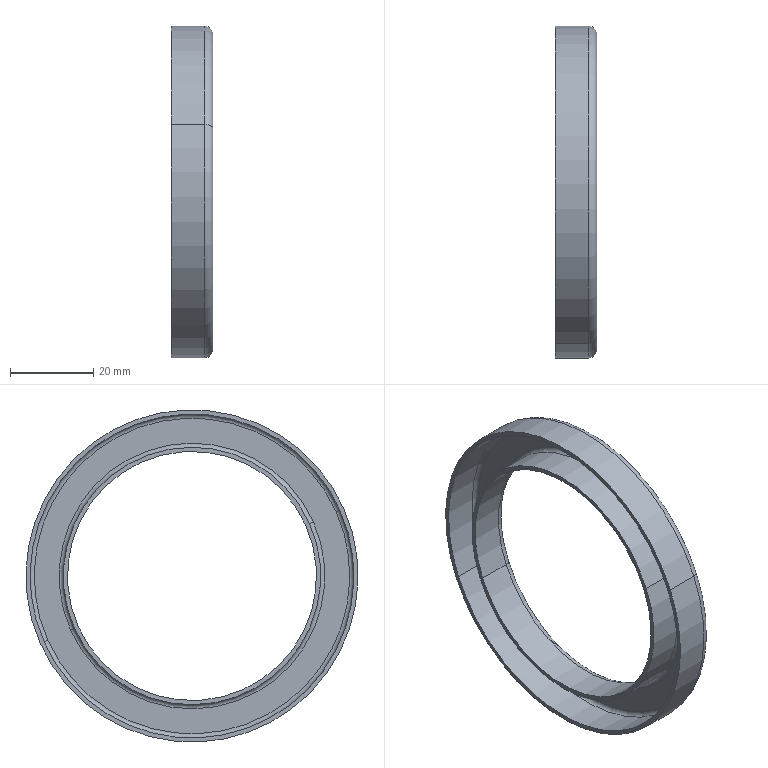Part | STEP file | Input 65 | 1 solid | 20 faces | box 10 x 80 x 80 mm | volume 5874 mm3 | cylinder 8 | torus 8 | plane 4 | commonest cylinder face diameters 60 x2 62 x2 78 x2 80 x2
STEP:
#1=CARTESIAN_POINT('',(0.,0.,0.));
#2=DIRECTION('',(0.,0.,1.));
#3=DIRECTION('',(1.,0.,0.));
#4=AXIS2_PLACEMENT_3D('',#1,#2,#3);
#5=CARTESIAN_POINT('',(4135.,-28.311,12.628));
#6=VERTEX_POINT('',#5);
#7=CARTESIAN_POINT('',(4135.,28.311,-12.628));
#8=VERTEX_POINT('',#7);
#9=CARTESIAN_POINT('',(4135.,0.,0.));
#10=DIRECTION('',(-1.,0.,0.));
#11=DIRECTION('',(0.,-0.9133,0.4074));
#12=AXIS2_PLACEMENT_3D('',#9,#10,#11);
#13=CIRCLE('',#12,31.);
#14=CARTESIAN_POINT('',(4127.,0.,0.));
#15=DIRECTION('',(-1.,0.,0.));
#16=DIRECTION('',(0.,-0.9133,0.4074));
#17=AXIS2_PLACEMENT_3D('',#14,#15,#16);
#18=CYLINDRICAL_SURFACE('',#17,31.);
#19=CARTESIAN_POINT('',(0.,-8.));
#20=DIRECTION('',(1.,0.));
#21=VECTOR('',#20,1.);
#22=LINE('',#19,#21);
#23=(GEOMETRIC_REPRESENTATION_CONTEXT(2)PARAMETRIC_REPRESENTATION_CONTEXT()REPRESENTATION_CONTEXT('',''));
#24=DEFINITIONAL_REPRESENTATION('',(#22),#23);
#25=PCURVE('',#18,#24);
#26=CARTESIAN_POINT('',(4135.,0.,0.));
#27=DIRECTION('',(-1.,0.,0.));
#28=DIRECTION('',(0.,-0.9133,0.4074));
#29=AXIS2_PLACEMENT_3D('',#26,#27,#28);
#30=TOROIDAL_SURFACE('',#29,32.,1.);
#31=CARTESIAN_POINT('',(0.,3.142));
#32=DIRECTION('',(1.,0.));
#33=VECTOR('',#32,1.);
#34=LINE('',#31,#33);
#35=(GEOMETRIC_REPRESENTATION_CONTEXT(2)PARAMETRIC_REPRESENTATION_CONTEXT()REPRESENTATION_CONTEXT('',''));
#36=DEFINITIONAL_REPRESENTATION('',(#34),#35);
#37=PCURVE('',#30,#36);
#38=SURFACE_CURVE('',#13,(#25,#37),.PCURVE_S1.);
#39=EDGE_CURVE('',#6,#8,#38,.T.);
#40=ORIENTED_EDGE('',*,*,#39,.T.);
#41=CARTESIAN_POINT('',(4127.,28.311,-12.628));
#42=VERTEX_POINT('',#41);
#43=CARTESIAN_POINT('',(4127.,28.311,-12.628));
#44=DIRECTION('',(-1.,0.,0.));
#45=VECTOR('',#44,1.);
#46=LINE('',#43,#45);
#47=CARTESIAN_POINT('',(3.142,0.));
#48=DIRECTION('',(0.,1.));
#49=VECTOR('',#48,1.);
#50=LINE('',#47,#49);
#51=(GEOMETRIC_REPRESENTATION_CONTEXT(2)PARAMETRIC_REPRESENTATION_CONTEXT()REPRESENTATION_CONTEXT('',''));
#52=DEFINITIONAL_REPRESENTATION('',(#50),#51);
#53=PCURVE('',#18,#52);
#54=CARTESIAN_POINT('',(4127.,0.,0.));
#55=DIRECTION('',(-1.,0.,0.));
#56=DIRECTION('',(0.,-0.9133,0.4074));
#57=AXIS2_PLACEMENT_3D('',#54,#55,#56);
#58=CYLINDRICAL_SURFACE('',#57,31.);
#59=CARTESIAN_POINT('',(3.142,0.));
#60=DIRECTION('',(0.,1.));
#61=VECTOR('',#60,1.);
#62=LINE('',#59,#61);
#63=(GEOMETRIC_REPRESENTATION_CONTEXT(2)PARAMETRIC_REPRESENTATION_CONTEXT()REPRESENTATION_CONTEXT('',''));
#64=DEFINITIONAL_REPRESENTATION('',(#62),#63);
#65=PCURVE('',#58,#64);
#66=SURFACE_CURVE('',#46,(#53,#65),.PCURVE_S1.);
#67=EDGE_CURVE('',#8,#42,#66,.T.);
#68=ORIENTED_EDGE('',*,*,#67,.T.);
#69=CARTESIAN_POINT('',(4127.,-28.311,12.628));
#70=VERTEX_POINT('',#69);
#71=CARTESIAN_POINT('',(4127.,0.,0.));
#72=DIRECTION('',(-1.,0.,0.));
#73=DIRECTION('',(0.,-0.9133,0.4074));
#74=AXIS2_PLACEMENT_3D('',#71,#72,#73);
#75=CIRCLE('',#74,31.);
#76=CARTESIAN_POINT('',(0.,0.));
#77=DIRECTION('',(1.,0.));
#78=VECTOR('',#77,1.);
#79=LINE('',#76,#78);
#80=(GEOMETRIC_REPRESENTATION_CONTEXT(2)PARAMETRIC_REPRESENTATION_CONTEXT()REPRESENTATION_CONTEXT('',''));
#81=DEFINITIONAL_REPRESENTATION('',(#79),#80);
#82=PCURVE('',#18,#81);
#83=CARTESIAN_POINT('',(4127.,-28.311,12.628));
#84=DIRECTION('',(-1.,0.,0.));
#85=DIRECTION('',(0.,-0.9133,0.4074));
#86=AXIS2_PLACEMENT_3D('',#83,#84,#85);
#87=PLANE('',#86);
#88=CARTESIAN_POINT('',(-31.,0.));
#89=DIRECTION('',(1.,0.));
#90=AXIS2_PLACEMENT_2D('',#88,#89);
#91=CIRCLE('',#90,31.);
#92=(GEOMETRIC_REPRESENTATION_CONTEXT(2)PARAMETRIC_REPRESENTATION_CONTEXT()REPRESENTATION_CONTEXT('',''));
#93=DEFINITIONAL_REPRESENTATION('',(#91),#92);
#94=PCURVE('',#87,#93);
#95=SURFACE_CURVE('',#75,(#82,#94),.PCURVE_S1.);
#96=EDGE_CURVE('',#70,#42,#95,.T.);
#97=ORIENTED_EDGE('',*,*,#96,.F.);
#98=CARTESIAN_POINT('',(4127.,-28.311,12.628));
#99=DIRECTION('',(-1.,0.,0.));
#100=VECTOR('',#99,1.);
#101=LINE('',#98,#100);
#102=CARTESIAN_POINT('',(0.,0.));
#103=DIRECTION('',(0.,1.));
#104=VECTOR('',#103,1.);
#105=LINE('',#102,#104);
#106=(GEOMETRIC_REPRESENTATION_CONTEXT(2)PARAMETRIC_REPRESENTATION_CONTEXT()REPRESENTATION_CONTEXT('',''));
#107=DEFINITIONAL_REPRESENTATION('',(#105),#106);
#108=PCURVE('',#18,#107);
#109=CARTESIAN_POINT('',(6.283,0.));
#110=DIRECTION('',(0.,1.));
#111=VECTOR('',#110,1.);
#112=LINE('',#109,#111);
#113=(GEOMETRIC_REPRESENTATION_CONTEXT(2)PARAMETRIC_REPRESENTATION_CONTEXT()REPRESENTATION_CONTEXT('',''));
#114=DEFINITIONAL_REPRESENTATION('',(#112),#113);
#115=PCURVE('',#58,#114);
#116=SURFACE_CURVE('',#101,(#108,#115),.PCURVE_S1.);
#117=EDGE_CURVE('',#6,#70,#116,.T.);
#118=ORIENTED_EDGE('',*,*,#117,.F.);
#119=EDGE_LOOP('',(#40,#68,#97,#118));
#120=FACE_BOUND('',#119,.T.);
#121=ADVANCED_FACE('',(#120),#18,.T.);
#122=CARTESIAN_POINT('',(4136.,-29.225,13.036));
#123=VERTEX_POINT('',#122);
#124=CARTESIAN_POINT('',(4135.,-29.225,13.036));
#125=DIRECTION('',(0.,-0.4074,-0.9133));
#126=DIRECTION('',(0.,0.9133,-0.4074));
#127=AXIS2_PLACEMENT_3D('',#124,#125,#126);
#128=CIRCLE('',#127,1.);
#129=CARTESIAN_POINT('',(4135.,0.,0.));
#130=DIRECTION('',(-1.,0.,0.));
#131=DIRECTION('',(0.,-0.9133,0.4074));
#132=AXIS2_PLACEMENT_3D('',#129,#130,#131);
#133=TOROIDAL_SURFACE('',#132,32.,1.);
#134=CARTESIAN_POINT('',(6.283,3.142));
#135=DIRECTION('',(0.,1.));
#136=VECTOR('',#135,1.);
#137=LINE('',#134,#136);
#138=(GEOMETRIC_REPRESENTATION_CONTEXT(2)PARAMETRIC_REPRESENTATION_CONTEXT()REPRESENTATION_CONTEXT('',''));
#139=DEFINITIONAL_REPRESENTATION('',(#137),#138);
#140=PCURVE('',#133,#139);
#141=CARTESIAN_POINT('',(0.,3.142));
#142=DIRECTION('',(0.,1.));
#143=VECTOR('',#142,1.);
#144=LINE('',#141,#143);
#145=(GEOMETRIC_REPRESENTATION_CONTEXT(2)PARAMETRIC_REPRESENTATION_CONTEXT()REPRESENTATION_CONTEXT('',''));
#146=DEFINITIONAL_REPRESENTATION('',(#144),#145);
#147=PCURVE('',#30,#146);
#148=SURFACE_CURVE('',#128,(#140,#147),.PCURVE_S1.);
#149=EDGE_CURVE('',#6,#123,#148,.T.);
#150=ORIENTED_EDGE('',*,*,#149,.T.);
#151=CARTESIAN_POINT('',(4136.,29.225,-13.036));
#152=VERTEX_POINT('',#151);
#153=CARTESIAN_POINT('',(4136.,0.,0.));
#154=DIRECTION('',(-1.,0.,0.));
#155=DIRECTION('',(0.,-0.9133,0.4074));
#156=AXIS2_PLACEMENT_3D('',#153,#154,#155);
#157=CIRCLE('',#156,32.);
#158=CARTESIAN_POINT('',(0.,4.712));
#159=DIRECTION('',(1.,0.));
#160=VECTOR('',#159,1.);
#161=LINE('',#158,#160);
#162=(GEOMETRIC_REPRESENTATION_CONTEXT(2)PARAMETRIC_REPRESENTATION_CONTEXT()REPRESENTATION_CONTEXT('',''));
#163=DEFINITIONAL_REPRESENTATION('',(#161),#162);
#164=PCURVE('',#133,#163);
#165=CARTESIAN_POINT('',(4136.,-34.704,15.48));
#166=DIRECTION('',(-1.,0.,0.));
#167=DIRECTION('',(0.,-0.9133,0.4074));
#168=AXIS2_PLACEMENT_3D('',#165,#166,#167);
#169=PLANE('',#168);
#170=CARTESIAN_POINT('',(-38.,0.));
#171=DIRECTION('',(1.,0.));
#172=AXIS2_PLACEMENT_2D('',#170,#171);
#173=CIRCLE('',#172,32.);
#174=(GEOMETRIC_REPRESENTATION_CONTEXT(2)PARAMETRIC_REPRESENTATION_CONTEXT()REPRESENTATION_CONTEXT('',''));
#175=DEFINITIONAL_REPRESENTATION('',(#173),#174);
#176=PCURVE('',#169,#175);
#177=SURFACE_CURVE('',#157,(#164,#176),.PCURVE_S1.);
#178=EDGE_CURVE('',#152,#123,#177,.T.);
#179=ORIENTED_EDGE('',*,*,#178,.F.);
#180=CARTESIAN_POINT('',(4135.,29.225,-13.036));
#181=DIRECTION('',(0.,0.4074,0.9133));
#182=DIRECTION('',(0.,-0.9133,0.4074));
#183=AXIS2_PLACEMENT_3D('',#180,#181,#182);
#184=CIRCLE('',#183,1.);
#185=CARTESIAN_POINT('',(3.142,3.142));
#186=DIRECTION('',(0.,1.));
#187=VECTOR('',#186,1.);
#188=LINE('',#185,#187);
#189=(GEOMETRIC_REPRESENTATION_CONTEXT(2)PARAMETRIC_REPRESENTATION_CONTEXT()REPRESENTATION_CONTEXT('',''));
#190=DEFINITIONAL_REPRESENTATION('',(#188),#189);
#191=PCURVE('',#133,#190);
#192=CARTESIAN_POINT('',(3.142,3.142));
#193=DIRECTION('',(0.,1.));
#194=VECTOR('',#193,1.);
#195=LINE('',#192,#194);
#196=(GEOMETRIC_REPRESENTATION_CONTEXT(2)PARAMETRIC_REPRESENTATION_CONTEXT()REPRESENTATION_CONTEXT('',''));
#197=DEFINITIONAL_REPRESENTATION('',(#195),#196);
#198=PCURVE('',#30,#197);
#199=SURFACE_CURVE('',#184,(#191,#198),.PCURVE_S1.);
#200=EDGE_CURVE('',#8,#152,#199,.T.);
#201=ORIENTED_EDGE('',*,*,#200,.F.);
#202=CARTESIAN_POINT('',(4135.,0.,0.));
#203=DIRECTION('',(-1.,0.,0.));
#204=DIRECTION('',(0.,-0.9133,0.4074));
#205=AXIS2_PLACEMENT_3D('',#202,#203,#204);
#206=CIRCLE('',#205,31.);
#207=CARTESIAN_POINT('',(0.,3.142));
#208=DIRECTION('',(1.,0.));
#209=VECTOR('',#208,1.);
#210=LINE('',#207,#209);
#211=(GEOMETRIC_REPRESENTATION_CONTEXT(2)PARAMETRIC_REPRESENTATION_CONTEXT()REPRESENTATION_CONTEXT('',''));
#212=DEFINITIONAL_REPRESENTATION('',(#210),#211);
#213=PCURVE('',#133,#212);
#214=CARTESIAN_POINT('',(0.,-8.));
#215=DIRECTION('',(1.,0.));
#216=VECTOR('',#215,1.);
#217=LINE('',#214,#216);
#218=(GEOMETRIC_REPRESENTATION_CONTEXT(2)PARAMETRIC_REPRESENTATION_CONTEXT()REPRESENTATION_CONTEXT('',''));
#219=DEFINITIONAL_REPRESENTATION('',(#217),#218);
#220=PCURVE('',#58,#219);
#221=SURFACE_CURVE('',#206,(#213,#220),.PCURVE_S1.);
#222=EDGE_CURVE('',#8,#6,#221,.T.);
#223=ORIENTED_EDGE('',*,*,#222,.T.);
#224=EDGE_LOOP('',(#150,#179,#201,#223));
#225=FACE_BOUND('',#224,.F.);
#226=ADVANCED_FACE('',(#225),#133,.F.);
#227=CARTESIAN_POINT('',(4136.,-34.704,15.48));
#228=VERTEX_POINT('',#227);
#229=CARTESIAN_POINT('',(4135.,-35.617,15.887));
#230=VERTEX_POINT('',#229);
#231=CARTESIAN_POINT('',(4135.,-34.704,15.48));
#232=DIRECTION('',(0.,-0.4074,-0.9133));
#233=DIRECTION('',(0.,0.9133,-0.4074));
#234=AXIS2_PLACEMENT_3D('',#231,#232,#233);
#235=CIRCLE('',#234,1.);
#236=CARTESIAN_POINT('',(4135.,0.,0.));
#237=DIRECTION('',(-1.,0.,0.));
#238=DIRECTION('',(0.,-0.9133,0.4074));
#239=AXIS2_PLACEMENT_3D('',#236,#237,#238);
#240=TOROIDAL_SURFACE('',#239,38.,1.);
#241=CARTESIAN_POINT('',(6.283,3.142));
#242=DIRECTION('',(0.,1.));
#243=VECTOR('',#242,1.);
#244=LINE('',#241,#243);
#245=(GEOMETRIC_REPRESENTATION_CONTEXT(2)PARAMETRIC_REPRESENTATION_CONTEXT()REPRESENTATION_CONTEXT('',''));
#246=DEFINITIONAL_REPRESENTATION('',(#244),#245);
#247=PCURVE('',#240,#246);
#248=CARTESIAN_POINT('',(4135.,0.,0.));
#249=DIRECTION('',(-1.,0.,0.));
#250=DIRECTION('',(0.,-0.9133,0.4074));
#251=AXIS2_PLACEMENT_3D('',#248,#249,#250);
#252=TOROIDAL_SURFACE('',#251,38.,1.);
#253=CARTESIAN_POINT('',(0.,3.142));
#254=DIRECTION('',(0.,1.));
#255=VECTOR('',#254,1.);
#256=LINE('',#253,#255);
#257=(GEOMETRIC_REPRESENTATION_CONTEXT(2)PARAMETRIC_REPRESENTATION_CONTEXT()REPRESENTATION_CONTEXT('',''));
#258=DEFINITIONAL_REPRESENTATION('',(#256),#257);
#259=PCURVE('',#252,#258);
#260=SURFACE_CURVE('',#235,(#247,#259),.PCURVE_S1.);
#261=EDGE_CURVE('',#228,#230,#260,.T.);
#262=ORIENTED_EDGE('',*,*,#261,.T.);
#263=CARTESIAN_POINT('',(4135.,35.617,-15.887));
#264=VERTEX_POINT('',#263);
#265=CARTESIAN_POINT('',(4135.,0.,0.));
#266=DIRECTION('',(-1.,0.,0.));
#267=DIRECTION('',(0.,-0.9133,0.4074));
#268=AXIS2_PLACEMENT_3D('',#265,#266,#267);
#269=CIRCLE('',#268,39.);
#270=CARTESIAN_POINT('',(0.,6.283));
#271=DIRECTION('',(1.,0.));
#272=VECTOR('',#271,1.);
#273=LINE('',#270,#272);
#274=(GEOMETRIC_REPRESENTATION_CONTEXT(2)PARAMETRIC_REPRESENTATION_CONTEXT()REPRESENTATION_CONTEXT('',''));
#275=DEFINITIONAL_REPRESENTATION('',(#273),#274);
#276=PCURVE('',#240,#275);
#277=CARTESIAN_POINT('',(4127.,0.,0.));
#278=DIRECTION('',(-1.,0.,0.));
#279=DIRECTION('',(0.,-0.9133,0.4074));
#280=AXIS2_PLACEMENT_3D('',#277,#278,#279);
#281=CYLINDRICAL_SURFACE('',#280,39.);
#282=CARTESIAN_POINT('',(0.,-8.));
#283=DIRECTION('',(1.,0.));
#284=VECTOR('',#283,1.);
#285=LINE('',#282,#284);
#286=(GEOMETRIC_REPRESENTATION_CONTEXT(2)PARAMETRIC_REPRESENTATION_CONTEXT()REPRESENTATION_CONTEXT('',''));
#287=DEFINITIONAL_REPRESENTATION('',(#285),#286);
#288=PCURVE('',#281,#287);
#289=SURFACE_CURVE('',#269,(#276,#288),.PCURVE_S1.);
#290=EDGE_CURVE('',#264,#230,#289,.T.);
#291=ORIENTED_EDGE('',*,*,#290,.F.);
#292=CARTESIAN_POINT('',(4136.,34.704,-15.48));
#293=VERTEX_POINT('',#292);
#294=CARTESIAN_POINT('',(4135.,34.704,-15.48));
#295=DIRECTION('',(0.,0.4074,0.9133));
#296=DIRECTION('',(0.,-0.9133,0.4074));
#297=AXIS2_PLACEMENT_3D('',#294,#295,#296);
#298=CIRCLE('',#297,1.);
#299=CARTESIAN_POINT('',(3.142,3.142));
#300=DIRECTION('',(0.,1.));
#301=VECTOR('',#300,1.);
#302=LINE('',#299,#301);
#303=(GEOMETRIC_REPRESENTATION_CONTEXT(2)PARAMETRIC_REPRESENTATION_CONTEXT()REPRESENTATION_CONTEXT('',''));
#304=DEFINITIONAL_REPRESENTATION('',(#302),#303);
#305=PCURVE('',#240,#304);
#306=CARTESIAN_POINT('',(3.142,3.142));
#307=DIRECTION('',(0.,1.));
#308=VECTOR('',#307,1.);
#309=LINE('',#306,#308);
#310=(GEOMETRIC_REPRESENTATION_CONTEXT(2)PARAMETRIC_REPRESENTATION_CONTEXT()REPRESENTATION_CONTEXT('',''));
#311=DEFINITIONAL_REPRESENTATION('',(#309),#310);
#312=PCURVE('',#252,#311);
#313=SURFACE_CURVE('',#298,(#305,#312),.PCURVE_S1.);
#314=EDGE_CURVE('',#293,#264,#313,.T.);
#315=ORIENTED_EDGE('',*,*,#314,.F.);
#316=CARTESIAN_POINT('',(4136.,0.,0.));
#317=DIRECTION('',(-1.,0.,0.));
#318=DIRECTION('',(0.,-0.9133,0.4074));
#319=AXIS2_PLACEMENT_3D('',#316,#317,#318);
#320=CIRCLE('',#319,38.);
#321=CARTESIAN_POINT('',(0.,4.712));
#322=DIRECTION('',(1.,0.));
#323=VECTOR('',#322,1.);
#324=LINE('',#321,#323);
#325=(GEOMETRIC_REPRESENTATION_CONTEXT(2)PARAMETRIC_REPRESENTATION_CONTEXT()REPRESENTATION_CONTEXT('',''));
#326=DEFINITIONAL_REPRESENTATION('',(#324),#325);
#327=PCURVE('',#240,#326);
#328=CARTESIAN_POINT('',(-38.,0.));
#329=DIRECTION('',(1.,0.));
#330=AXIS2_PLACEMENT_2D('',#328,#329);
#331=CIRCLE('',#330,38.);
#332=(GEOMETRIC_REPRESENTATION_CONTEXT(2)PARAMETRIC_REPRESENTATION_CONTEXT()REPRESENTATION_CONTEXT('',''));
#333=DEFINITIONAL_REPRESENTATION('',(#331),#332);
#334=PCURVE('',#169,#333);
#335=SURFACE_CURVE('',#320,(#327,#334),.PCURVE_S1.);
#336=EDGE_CURVE('',#293,#228,#335,.T.);
#337=ORIENTED_EDGE('',*,*,#336,.T.);
#338=EDGE_LOOP('',(#262,#291,#315,#337));
#339=FACE_BOUND('',#338,.F.);
#340=ADVANCED_FACE('',(#339),#240,.F.);
#341=CARTESIAN_POINT('',(4127.,-35.617,15.887));
#342=VERTEX_POINT('',#341);
#343=CARTESIAN_POINT('',(4127.,-35.617,15.887));
#344=DIRECTION('',(-1.,0.,0.));
#345=VECTOR('',#344,1.);
#346=LINE('',#343,#345);
#347=CARTESIAN_POINT('',(6.283,0.));
#348=DIRECTION('',(0.,1.));
#349=VECTOR('',#348,1.);
#350=LINE('',#347,#349);
#351=(GEOMETRIC_REPRESENTATION_CONTEXT(2)PARAMETRIC_REPRESENTATION_CONTEXT()REPRESENTATION_CONTEXT('',''));
#352=DEFINITIONAL_REPRESENTATION('',(#350),#351);
#353=PCURVE('',#281,#352);
#354=CARTESIAN_POINT('',(4127.,0.,0.));
#355=DIRECTION('',(-1.,0.,0.));
#356=DIRECTION('',(0.,-0.9133,0.4074));
#357=AXIS2_PLACEMENT_3D('',#354,#355,#356);
#358=CYLINDRICAL_SURFACE('',#357,39.);
#359=CARTESIAN_POINT('',(0.,0.));
#360=DIRECTION('',(0.,1.));
#361=VECTOR('',#360,1.);
#362=LINE('',#359,#361);
#363=(GEOMETRIC_REPRESENTATION_CONTEXT(2)PARAMETRIC_REPRESENTATION_CONTEXT()REPRESENTATION_CONTEXT('',''));
#364=DEFINITIONAL_REPRESENTATION('',(#362),#363);
#365=PCURVE('',#358,#364);
#366=SURFACE_CURVE('',#346,(#353,#365),.PCURVE_S1.);
#367=EDGE_CURVE('',#230,#342,#366,.T.);
#368=ORIENTED_EDGE('',*,*,#367,.T.);
#369=CARTESIAN_POINT('',(4127.,35.617,-15.887));
#370=VERTEX_POINT('',#369);
#371=CARTESIAN_POINT('',(4127.,0.,0.));
#372=DIRECTION('',(-1.,0.,0.));
#373=DIRECTION('',(0.,-0.9133,0.4074));
#374=AXIS2_PLACEMENT_3D('',#371,#372,#373);
#375=CIRCLE('',#374,39.);
#376=CARTESIAN_POINT('',(0.,0.));
#377=DIRECTION('',(1.,0.));
#378=VECTOR('',#377,1.);
#379=LINE('',#376,#378);
#380=(GEOMETRIC_REPRESENTATION_CONTEXT(2)PARAMETRIC_REPRESENTATION_CONTEXT()REPRESENTATION_CONTEXT('',''));
#381=DEFINITIONAL_REPRESENTATION('',(#379),#380);
#382=PCURVE('',#281,#381);
#383=CARTESIAN_POINT('',(4127.,-36.531,16.295));
#384=DIRECTION('',(-1.,0.,0.));
#385=DIRECTION('',(0.,-0.9133,0.4074));
#386=AXIS2_PLACEMENT_3D('',#383,#384,#385);
#387=PLANE('',#386);
#388=CARTESIAN_POINT('',(-40.,0.));
#389=DIRECTION('',(1.,0.));
#390=AXIS2_PLACEMENT_2D('',#388,#389);
#391=CIRCLE('',#390,39.);
#392=(GEOMETRIC_REPRESENTATION_CONTEXT(2)PARAMETRIC_REPRESENTATION_CONTEXT()REPRESENTATION_CONTEXT('',''));
#393=DEFINITIONAL_REPRESENTATION('',(#391),#392);
#394=PCURVE('',#387,#393);
#395=SURFACE_CURVE('',#375,(#382,#394),.PCURVE_S1.);
#396=EDGE_CURVE('',#370,#342,#395,.T.);
#397=ORIENTED_EDGE('',*,*,#396,.F.);
#398=CARTESIAN_POINT('',(4127.,35.617,-15.887));
#399=DIRECTION('',(-1.,0.,0.));
#400=VECTOR('',#399,1.);
#401=LINE('',#398,#400);
#402=CARTESIAN_POINT('',(3.142,0.));
#403=DIRECTION('',(0.,1.));
#404=VECTOR('',#403,1.);
#405=LINE('',#402,#404);
#406=(GEOMETRIC_REPRESENTATION_CONTEXT(2)PARAMETRIC_REPRESENTATION_CONTEXT()REPRESENTATION_CONTEXT('',''));
#407=DEFINITIONAL_REPRESENTATION('',(#405),#406);
#408=PCURVE('',#281,#407);
#409=CARTESIAN_POINT('',(3.142,0.));
#410=DIRECTION('',(0.,1.));
#411=VECTOR('',#410,1.);
#412=LINE('',#409,#411);
#413=(GEOMETRIC_REPRESENTATION_CONTEXT(2)PARAMETRIC_REPRESENTATION_CONTEXT()REPRESENTATION_CONTEXT('',''));
#414=DEFINITIONAL_REPRESENTATION('',(#412),#413);
#415=PCURVE('',#358,#414);
#416=SURFACE_CURVE('',#401,(#408,#415),.PCURVE_S1.);
#417=EDGE_CURVE('',#264,#370,#416,.T.);
#418=ORIENTED_EDGE('',*,*,#417,.F.);
#419=ORIENTED_EDGE('',*,*,#290,.T.);
#420=EDGE_LOOP('',(#368,#397,#418,#419));
#421=FACE_BOUND('',#420,.F.);
#422=ADVANCED_FACE('',(#421),#281,.F.);
#423=CARTESIAN_POINT('',(4135.,-36.531,16.295));
#424=VERTEX_POINT('',#423);
#425=CARTESIAN_POINT('',(4135.,36.531,-16.295));
#426=VERTEX_POINT('',#425);
#427=CARTESIAN_POINT('',(4135.,0.,0.));
#428=DIRECTION('',(-1.,0.,0.));
#429=DIRECTION('',(0.,-0.9133,0.4074));
#430=AXIS2_PLACEMENT_3D('',#427,#428,#429);
#431=CIRCLE('',#430,40.);
#432=CARTESIAN_POINT('',(4127.,0.,0.));
#433=DIRECTION('',(-1.,0.,0.));
#434=DIRECTION('',(0.,-0.9133,0.4074));
#435=AXIS2_PLACEMENT_3D('',#432,#433,#434);
#436=CYLINDRICAL_SURFACE('',#435,40.);
#437=CARTESIAN_POINT('',(0.,-8.));
#438=DIRECTION('',(1.,0.));
#439=VECTOR('',#438,1.);
#440=LINE('',#437,#439);
#441=(GEOMETRIC_REPRESENTATION_CONTEXT(2)PARAMETRIC_REPRESENTATION_CONTEXT()REPRESENTATION_CONTEXT('',''));
#442=DEFINITIONAL_REPRESENTATION('',(#440),#441);
#443=PCURVE('',#436,#442);
#444=CARTESIAN_POINT('',(4135.,0.,0.));
#445=DIRECTION('',(-1.,0.,0.));
#446=DIRECTION('',(0.,-0.9133,0.4074));
#447=AXIS2_PLACEMENT_3D('',#444,#445,#446);
#448=TOROIDAL_SURFACE('',#447,38.,2.);
#449=CARTESIAN_POINT('',(0.,6.283));
#450=DIRECTION('',(1.,0.));
#451=VECTOR('',#450,1.);
#452=LINE('',#449,#451);
#453=(GEOMETRIC_REPRESENTATION_CONTEXT(2)PARAMETRIC_REPRESENTATION_CONTEXT()REPRESENTATION_CONTEXT('',''));
#454=DEFINITIONAL_REPRESENTATION('',(#452),#453);
#455=PCURVE('',#448,#454);
#456=SURFACE_CURVE('',#431,(#443,#455),.PCURVE_S1.);
#457=EDGE_CURVE('',#424,#426,#456,.T.);
#458=ORIENTED_EDGE('',*,*,#457,.T.);
#459=CARTESIAN_POINT('',(4127.,36.531,-16.295));
#460=VERTEX_POINT('',#459);
#461=CARTESIAN_POINT('',(4127.,36.531,-16.295));
#462=DIRECTION('',(-1.,0.,0.));
#463=VECTOR('',#462,1.);
#464=LINE('',#461,#463);
#465=CARTESIAN_POINT('',(3.142,0.));
#466=DIRECTION('',(0.,1.));
#467=VECTOR('',#466,1.);
#468=LINE('',#465,#467);
#469=(GEOMETRIC_REPRESENTATION_CONTEXT(2)PARAMETRIC_REPRESENTATION_CONTEXT()REPRESENTATION_CONTEXT('',''));
#470=DEFINITIONAL_REPRESENTATION('',(#468),#469);
#471=PCURVE('',#436,#470);
#472=CARTESIAN_POINT('',(4127.,0.,0.));
#473=DIRECTION('',(-1.,0.,0.));
#474=DIRECTION('',(0.,-0.9133,0.4074));
#475=AXIS2_PLACEMENT_3D('',#472,#473,#474);
#476=CYLINDRICAL_SURFACE('',#475,40.);
#477=CARTESIAN_POINT('',(3.142,0.));
#478=DIRECTION('',(0.,1.));
#479=VECTOR('',#478,1.);
#480=LINE('',#477,#479);
#481=(GEOMETRIC_REPRESENTATION_CONTEXT(2)PARAMETRIC_REPRESENTATION_CONTEXT()REPRESENTATION_CONTEXT('',''));
#482=DEFINITIONAL_REPRESENTATION('',(#480),#481);
#483=PCURVE('',#476,#482);
#484=SURFACE_CURVE('',#464,(#471,#483),.PCURVE_S1.);
#485=EDGE_CURVE('',#426,#460,#484,.T.);
#486=ORIENTED_EDGE('',*,*,#485,.T.);
#487=CARTESIAN_POINT('',(4127.,-36.531,16.295));
#488=VERTEX_POINT('',#487);
#489=CARTESIAN_POINT('',(4127.,0.,0.));
#490=DIRECTION('',(-1.,0.,0.));
#491=DIRECTION('',(0.,-0.9133,0.4074));
#492=AXIS2_PLACEMENT_3D('',#489,#490,#491);
#493=CIRCLE('',#492,40.);
#494=CARTESIAN_POINT('',(0.,0.));
#495=DIRECTION('',(1.,0.));
#496=VECTOR('',#495,1.);
#497=LINE('',#494,#496);
#498=(GEOMETRIC_REPRESENTATION_CONTEXT(2)PARAMETRIC_REPRESENTATION_CONTEXT()REPRESENTATION_CONTEXT('',''));
#499=DEFINITIONAL_REPRESENTATION('',(#497),#498);
#500=PCURVE('',#436,#499);
#501=CARTESIAN_POINT('',(-40.,0.));
#502=DIRECTION('',(1.,0.));
#503=AXIS2_PLACEMENT_2D('',#501,#502);
#504=CIRCLE('',#503,40.);
#505=(GEOMETRIC_REPRESENTATION_CONTEXT(2)PARAMETRIC_REPRESENTATION_CONTEXT()REPRESENTATION_CONTEXT('',''));
#506=DEFINITIONAL_REPRESENTATION('',(#504),#505);
#507=PCURVE('',#387,#506);
#508=SURFACE_CURVE('',#493,(#500,#507),.PCURVE_S1.);
#509=EDGE_CURVE('',#488,#460,#508,.T.);
#510=ORIENTED_EDGE('',*,*,#509,.F.);
#511=CARTESIAN_POINT('',(4127.,-36.531,16.295));
#512=DIRECTION('',(-1.,0.,0.));
#513=VECTOR('',#512,1.);
#514=LINE('',#511,#513);
#515=CARTESIAN_POINT('',(0.,0.));
#516=DIRECTION('',(0.,1.));
#517=VECTOR('',#516,1.);
#518=LINE('',#515,#517);
#519=(GEOMETRIC_REPRESENTATION_CONTEXT(2)PARAMETRIC_REPRESENTATION_CONTEXT()REPRESENTATION_CONTEXT('',''));
#520=DEFINITIONAL_REPRESENTATION('',(#518),#519);
#521=PCURVE('',#436,#520);
#522=CARTESIAN_POINT('',(6.283,0.));
#523=DIRECTION('',(0.,1.));
#524=VECTOR('',#523,1.);
#525=LINE('',#522,#524);
#526=(GEOMETRIC_REPRESENTATION_CONTEXT(2)PARAMETRIC_REPRESENTATION_CONTEXT()REPRESENTATION_CONTEXT('',''));
#527=DEFINITIONAL_REPRESENTATION('',(#525),#526);
#528=PCURVE('',#476,#527);
#529=SURFACE_CURVE('',#514,(#521,#528),.PCURVE_S1.);
#530=EDGE_CURVE('',#424,#488,#529,.T.);
#531=ORIENTED_EDGE('',*,*,#530,.F.);
#532=EDGE_LOOP('',(#458,#486,#510,#531));
#533=FACE_BOUND('',#532,.T.);
#534=ADVANCED_FACE('',(#533),#436,.T.);
#535=CARTESIAN_POINT('',(4137.,-34.704,15.48));
#536=VERTEX_POINT('',#535);
#537=CARTESIAN_POINT('',(4137.,34.704,-15.48));
#538=VERTEX_POINT('',#537);
#539=CARTESIAN_POINT('',(4137.,0.,0.));
#540=DIRECTION('',(-1.,0.,0.));
#541=DIRECTION('',(0.,-0.9133,0.4074));
#542=AXIS2_PLACEMENT_3D('',#539,#540,#541);
#543=CIRCLE('',#542,38.);
#544=CARTESIAN_POINT('',(0.,4.712));
#545=DIRECTION('',(1.,0.));
#546=VECTOR('',#545,1.);
#547=LINE('',#544,#546);
#548=(GEOMETRIC_REPRESENTATION_CONTEXT(2)PARAMETRIC_REPRESENTATION_CONTEXT()REPRESENTATION_CONTEXT('',''));
#549=DEFINITIONAL_REPRESENTATION('',(#547),#548);
#550=PCURVE('',#448,#549);
#551=CARTESIAN_POINT('',(4137.,-29.225,13.036));
#552=DIRECTION('',(1.,0.,0.));
#553=DIRECTION('',(0.,0.9133,-0.4074));
#554=AXIS2_PLACEMENT_3D('',#551,#552,#553);
#555=PLANE('',#554);
#556=CARTESIAN_POINT('',(-6.,0.));
#557=CARTESIAN_POINT('',(-6.,65.818));
#558=CARTESIAN_POINT('',(51.,32.909));
#559=CARTESIAN_POINT('',(108.,0.));
#560=CARTESIAN_POINT('',(51.,-32.909));
#561=CARTESIAN_POINT('',(-6.,-65.818));
#562=CARTESIAN_POINT('',(-6.,0.));
#563=(BOUNDED_CURVE()B_SPLINE_CURVE(2,(#556,#557,#558,#559,#560,#561,#562),.UNSPECIFIED.,.T.,.F.)B_SPLINE_CURVE_WITH_KNOTS((1,2,2,2,2,1),(-2.094,0.,2.094,4.189,6.283,8.378),.UNSPECIFIED.)CURVE()GEOMETRIC_REPRESENTATION_ITEM()RATIONAL_B_SPLINE_CURVE((1.,0.5,1.,0.5,1.,0.5,1.))REPRESENTATION_ITEM(''));
#564=(GEOMETRIC_REPRESENTATION_CONTEXT(2)PARAMETRIC_REPRESENTATION_CONTEXT()REPRESENTATION_CONTEXT('',''));
#565=DEFINITIONAL_REPRESENTATION('',(#563),#564);
#566=PCURVE('',#555,#565);
#567=SURFACE_CURVE('',#543,(#550,#566),.PCURVE_S1.);
#568=EDGE_CURVE('',#536,#538,#567,.T.);
#569=ORIENTED_EDGE('',*,*,#568,.T.);
#570=CARTESIAN_POINT('',(4135.,34.704,-15.48));
#571=DIRECTION('',(0.,0.4074,0.9133));
#572=DIRECTION('',(0.,-0.9133,0.4074));
#573=AXIS2_PLACEMENT_3D('',#570,#571,#572);
#574=CIRCLE('',#573,2.);
#575=CARTESIAN_POINT('',(3.142,3.142));
#576=DIRECTION('',(0.,1.));
#577=VECTOR('',#576,1.);
#578=LINE('',#575,#577);
#579=(GEOMETRIC_REPRESENTATION_CONTEXT(2)PARAMETRIC_REPRESENTATION_CONTEXT()REPRESENTATION_CONTEXT('',''));
#580=DEFINITIONAL_REPRESENTATION('',(#578),#579);
#581=PCURVE('',#448,#580);
#582=CARTESIAN_POINT('',(4135.,0.,0.));
#583=DIRECTION('',(-1.,0.,0.));
#584=DIRECTION('',(0.,-0.9133,0.4074));
#585=AXIS2_PLACEMENT_3D('',#582,#583,#584);
#586=TOROIDAL_SURFACE('',#585,38.,2.);
#587=CARTESIAN_POINT('',(3.142,3.142));
#588=DIRECTION('',(0.,1.));
#589=VECTOR('',#588,1.);
#590=LINE('',#587,#589);
#591=(GEOMETRIC_REPRESENTATION_CONTEXT(2)PARAMETRIC_REPRESENTATION_CONTEXT()REPRESENTATION_CONTEXT('',''));
#592=DEFINITIONAL_REPRESENTATION('',(#590),#591);
#593=PCURVE('',#586,#592);
#594=SURFACE_CURVE('',#574,(#581,#593),.PCURVE_S1.);
#595=EDGE_CURVE('',#538,#426,#594,.T.);
#596=ORIENTED_EDGE('',*,*,#595,.T.);
#597=ORIENTED_EDGE('',*,*,#457,.F.);
#598=CARTESIAN_POINT('',(4135.,-34.704,15.48));
#599=DIRECTION('',(0.,-0.4074,-0.9133));
#600=DIRECTION('',(0.,0.9133,-0.4074));
#601=AXIS2_PLACEMENT_3D('',#598,#599,#600);
#602=CIRCLE('',#601,2.);
#603=CARTESIAN_POINT('',(0.,3.142));
#604=DIRECTION('',(0.,1.));
#605=VECTOR('',#604,1.);
#606=LINE('',#603,#605);
#607=(GEOMETRIC_REPRESENTATION_CONTEXT(2)PARAMETRIC_REPRESENTATION_CONTEXT()REPRESENTATION_CONTEXT('',''));
#608=DEFINITIONAL_REPRESENTATION('',(#606),#607);
#609=PCURVE('',#448,#608);
#610=CARTESIAN_POINT('',(6.283,3.142));
#611=DIRECTION('',(0.,1.));
#612=VECTOR('',#611,1.);
#613=LINE('',#610,#612);
#614=(GEOMETRIC_REPRESENTATION_CONTEXT(2)PARAMETRIC_REPRESENTATION_CONTEXT()REPRESENTATION_CONTEXT('',''));
#615=DEFINITIONAL_REPRESENTATION('',(#613),#614);
#616=PCURVE('',#586,#615);
#617=SURFACE_CURVE('',#602,(#609,#616),.PCURVE_S1.);
#618=EDGE_CURVE('',#536,#424,#617,.T.);
#619=ORIENTED_EDGE('',*,*,#618,.F.);
#620=EDGE_LOOP('',(#569,#596,#597,#619));
#621=FACE_BOUND('',#620,.T.);
#622=ADVANCED_FACE('',(#621),#448,.T.);
#623=CARTESIAN_POINT('',(4135.,-27.398,12.221));
#624=VERTEX_POINT('',#623);
#625=CARTESIAN_POINT('',(4135.,27.398,-12.221));
#626=VERTEX_POINT('',#625);
#627=CARTESIAN_POINT('',(4135.,0.,0.));
#628=DIRECTION('',(-1.,0.,0.));
#629=DIRECTION('',(0.,-0.9133,0.4074));
#630=AXIS2_PLACEMENT_3D('',#627,#628,#629);
#631=CIRCLE('',#630,30.);
#632=CARTESIAN_POINT('',(4135.,0.,0.));
#633=DIRECTION('',(-1.,0.,0.));
#634=DIRECTION('',(0.,-0.9133,0.4074));
#635=AXIS2_PLACEMENT_3D('',#632,#633,#634);
#636=TOROIDAL_SURFACE('',#635,32.,2.);
#637=CARTESIAN_POINT('',(0.,3.142));
#638=DIRECTION('',(1.,0.));
#639=VECTOR('',#638,1.);
#640=LINE('',#637,#639);
#641=(GEOMETRIC_REPRESENTATION_CONTEXT(2)PARAMETRIC_REPRESENTATION_CONTEXT()REPRESENTATION_CONTEXT('',''));
#642=DEFINITIONAL_REPRESENTATION('',(#640),#641);
#643=PCURVE('',#636,#642);
#644=CARTESIAN_POINT('',(4127.,0.,0.));
#645=DIRECTION('',(-1.,0.,0.));
#646=DIRECTION('',(0.,-0.9133,0.4074));
#647=AXIS2_PLACEMENT_3D('',#644,#645,#646);
#648=CYLINDRICAL_SURFACE('',#647,30.);
#649=CARTESIAN_POINT('',(0.,-8.));
#650=DIRECTION('',(1.,0.));
#651=VECTOR('',#650,1.);
#652=LINE('',#649,#651);
#653=(GEOMETRIC_REPRESENTATION_CONTEXT(2)PARAMETRIC_REPRESENTATION_CONTEXT()REPRESENTATION_CONTEXT('',''));
#654=DEFINITIONAL_REPRESENTATION('',(#652),#653);
#655=PCURVE('',#648,#654);
#656=SURFACE_CURVE('',#631,(#643,#655),.PCURVE_S1.);
#657=EDGE_CURVE('',#624,#626,#656,.T.);
#658=ORIENTED_EDGE('',*,*,#657,.T.);
#659=CARTESIAN_POINT('',(4137.,29.225,-13.036));
#660=VERTEX_POINT('',#659);
#661=CARTESIAN_POINT('',(4135.,29.225,-13.036));
#662=DIRECTION('',(0.,0.4074,0.9133));
#663=DIRECTION('',(0.,-0.9133,0.4074));
#664=AXIS2_PLACEMENT_3D('',#661,#662,#663);
#665=CIRCLE('',#664,2.);
#666=CARTESIAN_POINT('',(3.142,3.142));
#667=DIRECTION('',(0.,1.));
#668=VECTOR('',#667,1.);
#669=LINE('',#666,#668);
#670=(GEOMETRIC_REPRESENTATION_CONTEXT(2)PARAMETRIC_REPRESENTATION_CONTEXT()REPRESENTATION_CONTEXT('',''));
#671=DEFINITIONAL_REPRESENTATION('',(#669),#670);
#672=PCURVE('',#636,#671);
#673=CARTESIAN_POINT('',(4135.,0.,0.));
#674=DIRECTION('',(-1.,0.,0.));
#675=DIRECTION('',(0.,-0.9133,0.4074));
#676=AXIS2_PLACEMENT_3D('',#673,#674,#675);
#677=TOROIDAL_SURFACE('',#676,32.,2.);
#678=CARTESIAN_POINT('',(3.142,3.142));
#679=DIRECTION('',(0.,1.));
#680=VECTOR('',#679,1.);
#681=LINE('',#678,#680);
#682=(GEOMETRIC_REPRESENTATION_CONTEXT(2)PARAMETRIC_REPRESENTATION_CONTEXT()REPRESENTATION_CONTEXT('',''));
#683=DEFINITIONAL_REPRESENTATION('',(#681),#682);
#684=PCURVE('',#677,#683);
#685=SURFACE_CURVE('',#665,(#672,#684),.PCURVE_S1.);
#686=EDGE_CURVE('',#626,#660,#685,.T.);
#687=ORIENTED_EDGE('',*,*,#686,.T.);
#688=CARTESIAN_POINT('',(4137.,-29.225,13.036));
#689=VERTEX_POINT('',#688);
#690=CARTESIAN_POINT('',(4137.,0.,0.));
#691=DIRECTION('',(-1.,0.,0.));
#692=DIRECTION('',(0.,-0.9133,0.4074));
#693=AXIS2_PLACEMENT_3D('',#690,#691,#692);
#694=CIRCLE('',#693,32.);
#695=CARTESIAN_POINT('',(0.,4.712));
#696=DIRECTION('',(1.,0.));
#697=VECTOR('',#696,1.);
#698=LINE('',#695,#697);
#699=(GEOMETRIC_REPRESENTATION_CONTEXT(2)PARAMETRIC_REPRESENTATION_CONTEXT()REPRESENTATION_CONTEXT('',''));
#700=DEFINITIONAL_REPRESENTATION('',(#698),#699);
#701=PCURVE('',#636,#700);
#702=CARTESIAN_POINT('',(0.,0.));
#703=CARTESIAN_POINT('',(0.,55.426));
#704=CARTESIAN_POINT('',(48.,27.713));
#705=CARTESIAN_POINT('',(96.,0.));
#706=CARTESIAN_POINT('',(48.,-27.713));
#707=CARTESIAN_POINT('',(0.,-55.426));
#708=CARTESIAN_POINT('',(0.,0.));
#709=(BOUNDED_CURVE()B_SPLINE_CURVE(2,(#702,#703,#704,#705,#706,#707,#708),.UNSPECIFIED.,.T.,.F.)B_SPLINE_CURVE_WITH_KNOTS((1,2,2,2,2,1),(-2.094,0.,2.094,4.189,6.283,8.378),.UNSPECIFIED.)CURVE()GEOMETRIC_REPRESENTATION_ITEM()RATIONAL_B_SPLINE_CURVE((1.,0.5,1.,0.5,1.,0.5,1.))REPRESENTATION_ITEM(''));
#710=(GEOMETRIC_REPRESENTATION_CONTEXT(2)PARAMETRIC_REPRESENTATION_CONTEXT()REPRESENTATION_CONTEXT('',''));
#711=DEFINITIONAL_REPRESENTATION('',(#709),#710);
#712=PCURVE('',#555,#711);
#713=SURFACE_CURVE('',#694,(#701,#712),.PCURVE_S1.);
#714=EDGE_CURVE('',#689,#660,#713,.T.);
#715=ORIENTED_EDGE('',*,*,#714,.F.);
#716=CARTESIAN_POINT('',(4135.,-29.225,13.036));
#717=DIRECTION('',(0.,-0.4074,-0.9133));
#718=DIRECTION('',(0.,0.9133,-0.4074));
#719=AXIS2_PLACEMENT_3D('',#716,#717,#718);
#720=CIRCLE('',#719,2.);
#721=CARTESIAN_POINT('',(0.,3.142));
#722=DIRECTION('',(0.,1.));
#723=VECTOR('',#722,1.);
#724=LINE('',#721,#723);
#725=(GEOMETRIC_REPRESENTATION_CONTEXT(2)PARAMETRIC_REPRESENTATION_CONTEXT()REPRESENTATION_CONTEXT('',''));
#726=DEFINITIONAL_REPRESENTATION('',(#724),#725);
#727=PCURVE('',#636,#726);
#728=CARTESIAN_POINT('',(6.283,3.142));
#729=DIRECTION('',(0.,1.));
#730=VECTOR('',#729,1.);
#731=LINE('',#728,#730);
#732=(GEOMETRIC_REPRESENTATION_CONTEXT(2)PARAMETRIC_REPRESENTATION_CONTEXT()REPRESENTATION_CONTEXT('',''));
#733=DEFINITIONAL_REPRESENTATION('',(#731),#732);
#734=PCURVE('',#677,#733);
#735=SURFACE_CURVE('',#720,(#727,#734),.PCURVE_S1.);
#736=EDGE_CURVE('',#624,#689,#735,.T.);
#737=ORIENTED_EDGE('',*,*,#736,.F.);
#738=EDGE_LOOP('',(#658,#687,#715,#737));
#739=FACE_BOUND('',#738,.T.);
#740=ADVANCED_FACE('',(#739),#636,.T.);
#741=CARTESIAN_POINT('',(4127.,-27.398,12.221));
#742=VERTEX_POINT('',#741);
#743=CARTESIAN_POINT('',(4127.,-27.398,12.221));
#744=DIRECTION('',(-1.,0.,0.));
#745=VECTOR('',#744,1.);
#746=LINE('',#743,#745);
#747=CARTESIAN_POINT('',(4127.,0.,0.));
#748=DIRECTION('',(-1.,0.,0.));
#749=DIRECTION('',(0.,-0.9133,0.4074));
#750=AXIS2_PLACEMENT_3D('',#747,#748,#749);
#751=CYLINDRICAL_SURFACE('',#750,30.);
#752=CARTESIAN_POINT('',(6.283,0.));
#753=DIRECTION('',(0.,1.));
#754=VECTOR('',#753,1.);
#755=LINE('',#752,#754);
#756=(GEOMETRIC_REPRESENTATION_CONTEXT(2)PARAMETRIC_REPRESENTATION_CONTEXT()REPRESENTATION_CONTEXT('',''));
#757=DEFINITIONAL_REPRESENTATION('',(#755),#756);
#758=PCURVE('',#751,#757);
#759=CARTESIAN_POINT('',(0.,0.));
#760=DIRECTION('',(0.,1.));
#761=VECTOR('',#760,1.);
#762=LINE('',#759,#761);
#763=(GEOMETRIC_REPRESENTATION_CONTEXT(2)PARAMETRIC_REPRESENTATION_CONTEXT()REPRESENTATION_CONTEXT('',''));
#764=DEFINITIONAL_REPRESENTATION('',(#762),#763);
#765=PCURVE('',#648,#764);
#766=SURFACE_CURVE('',#746,(#758,#765),.PCURVE_S1.);
#767=EDGE_CURVE('',#624,#742,#766,.T.);
#768=ORIENTED_EDGE('',*,*,#767,.T.);
#769=CARTESIAN_POINT('',(4127.,27.398,-12.221));
#770=VERTEX_POINT('',#769);
#771=CARTESIAN_POINT('',(4127.,0.,0.));
#772=DIRECTION('',(-1.,0.,0.));
#773=DIRECTION('',(0.,-0.9133,0.4074));
#774=AXIS2_PLACEMENT_3D('',#771,#772,#773);
#775=CIRCLE('',#774,30.);
#776=CARTESIAN_POINT('',(0.,0.));
#777=DIRECTION('',(1.,0.));
#778=VECTOR('',#777,1.);
#779=LINE('',#776,#778);
#780=(GEOMETRIC_REPRESENTATION_CONTEXT(2)PARAMETRIC_REPRESENTATION_CONTEXT()REPRESENTATION_CONTEXT('',''));
#781=DEFINITIONAL_REPRESENTATION('',(#779),#780);
#782=PCURVE('',#751,#781);
#783=CARTESIAN_POINT('',(-31.,0.));
#784=DIRECTION('',(1.,0.));
#785=AXIS2_PLACEMENT_2D('',#783,#784);
#786=CIRCLE('',#785,30.);
#787=(GEOMETRIC_REPRESENTATION_CONTEXT(2)PARAMETRIC_REPRESENTATION_CONTEXT()REPRESENTATION_CONTEXT('',''));
#788=DEFINITIONAL_REPRESENTATION('',(#786),#787);
#789=PCURVE('',#87,#788);
#790=SURFACE_CURVE('',#775,(#782,#789),.PCURVE_S1.);
#791=EDGE_CURVE('',#770,#742,#790,.T.);
#792=ORIENTED_EDGE('',*,*,#791,.F.);
#793=CARTESIAN_POINT('',(4127.,27.398,-12.221));
#794=DIRECTION('',(-1.,0.,0.));
#795=VECTOR('',#794,1.);
#796=LINE('',#793,#795);
#797=CARTESIAN_POINT('',(3.142,0.));
#798=DIRECTION('',(0.,1.));
#799=VECTOR('',#798,1.);
#800=LINE('',#797,#799);
#801=(GEOMETRIC_REPRESENTATION_CONTEXT(2)PARAMETRIC_REPRESENTATION_CONTEXT()REPRESENTATION_CONTEXT('',''));
#802=DEFINITIONAL_REPRESENTATION('',(#800),#801);
#803=PCURVE('',#751,#802);
#804=CARTESIAN_POINT('',(3.142,0.));
#805=DIRECTION('',(0.,1.));
#806=VECTOR('',#805,1.);
#807=LINE('',#804,#806);
#808=(GEOMETRIC_REPRESENTATION_CONTEXT(2)PARAMETRIC_REPRESENTATION_CONTEXT()REPRESENTATION_CONTEXT('',''));
#809=DEFINITIONAL_REPRESENTATION('',(#807),#808);
#810=PCURVE('',#648,#809);
#811=SURFACE_CURVE('',#796,(#803,#810),.PCURVE_S1.);
#812=EDGE_CURVE('',#626,#770,#811,.T.);
#813=ORIENTED_EDGE('',*,*,#812,.F.);
#814=CARTESIAN_POINT('',(4135.,0.,0.));
#815=DIRECTION('',(-1.,0.,0.));
#816=DIRECTION('',(0.,-0.9133,0.4074));
#817=AXIS2_PLACEMENT_3D('',#814,#815,#816);
#818=CIRCLE('',#817,30.);
#819=CARTESIAN_POINT('',(0.,-8.));
#820=DIRECTION('',(1.,0.));
#821=VECTOR('',#820,1.);
#822=LINE('',#819,#821);
#823=(GEOMETRIC_REPRESENTATION_CONTEXT(2)PARAMETRIC_REPRESENTATION_CONTEXT()REPRESENTATION_CONTEXT('',''));
#824=DEFINITIONAL_REPRESENTATION('',(#822),#823);
#825=PCURVE('',#751,#824);
#826=CARTESIAN_POINT('',(0.,3.142));
#827=DIRECTION('',(1.,0.));
#828=VECTOR('',#827,1.);
#829=LINE('',#826,#828);
#830=(GEOMETRIC_REPRESENTATION_CONTEXT(2)PARAMETRIC_REPRESENTATION_CONTEXT()REPRESENTATION_CONTEXT('',''));
#831=DEFINITIONAL_REPRESENTATION('',(#829),#830);
#832=PCURVE('',#677,#831);
#833=SURFACE_CURVE('',#818,(#825,#832),.PCURVE_S1.);
#834=EDGE_CURVE('',#626,#624,#833,.T.);
#835=ORIENTED_EDGE('',*,*,#834,.T.);
#836=EDGE_LOOP('',(#768,#792,#813,#835));
#837=FACE_BOUND('',#836,.F.);
#838=ADVANCED_FACE('',(#837),#751,.F.);
#839=ORIENTED_EDGE('',*,*,#96,.T.);
#840=CARTESIAN_POINT('',(4127.,0.,0.));
#841=DIRECTION('',(-1.,0.,0.));
#842=DIRECTION('',(0.,-0.9133,0.4074));
#843=AXIS2_PLACEMENT_3D('',#840,#841,#842);
#844=CIRCLE('',#843,31.);
#845=CARTESIAN_POINT('',(-31.,0.));
#846=DIRECTION('',(1.,0.));
#847=AXIS2_PLACEMENT_2D('',#845,#846);
#848=CIRCLE('',#847,31.);
#849=(GEOMETRIC_REPRESENTATION_CONTEXT(2)PARAMETRIC_REPRESENTATION_CONTEXT()REPRESENTATION_CONTEXT('',''));
#850=DEFINITIONAL_REPRESENTATION('',(#848),#849);
#851=PCURVE('',#87,#850);
#852=CARTESIAN_POINT('',(0.,0.));
#853=DIRECTION('',(1.,0.));
#854=VECTOR('',#853,1.);
#855=LINE('',#852,#854);
#856=(GEOMETRIC_REPRESENTATION_CONTEXT(2)PARAMETRIC_REPRESENTATION_CONTEXT()REPRESENTATION_CONTEXT('',''));
#857=DEFINITIONAL_REPRESENTATION('',(#855),#856);
#858=PCURVE('',#58,#857);
#859=SURFACE_CURVE('',#844,(#851,#858),.PCURVE_S1.);
#860=EDGE_CURVE('',#42,#70,#859,.T.);
#861=ORIENTED_EDGE('',*,*,#860,.T.);
#862=EDGE_LOOP('',(#839,#861));
#863=FACE_BOUND('',#862,.T.);
#864=CARTESIAN_POINT('',(4127.,0.,0.));
#865=DIRECTION('',(-1.,0.,0.));
#866=DIRECTION('',(0.,-0.9133,0.4074));
#867=AXIS2_PLACEMENT_3D('',#864,#865,#866);
#868=CIRCLE('',#867,30.);
#869=CARTESIAN_POINT('',(-31.,0.));
#870=DIRECTION('',(1.,0.));
#871=AXIS2_PLACEMENT_2D('',#869,#870);
#872=CIRCLE('',#871,30.);
#873=(GEOMETRIC_REPRESENTATION_CONTEXT(2)PARAMETRIC_REPRESENTATION_CONTEXT()REPRESENTATION_CONTEXT('',''));
#874=DEFINITIONAL_REPRESENTATION('',(#872),#873);
#875=PCURVE('',#87,#874);
#876=CARTESIAN_POINT('',(0.,0.));
#877=DIRECTION('',(1.,0.));
#878=VECTOR('',#877,1.);
#879=LINE('',#876,#878);
#880=(GEOMETRIC_REPRESENTATION_CONTEXT(2)PARAMETRIC_REPRESENTATION_CONTEXT()REPRESENTATION_CONTEXT('',''));
#881=DEFINITIONAL_REPRESENTATION('',(#879),#880);
#882=PCURVE('',#648,#881);
#883=SURFACE_CURVE('',#868,(#875,#882),.PCURVE_S1.);
#884=EDGE_CURVE('',#742,#770,#883,.T.);
#885=ORIENTED_EDGE('',*,*,#884,.F.);
#886=ORIENTED_EDGE('',*,*,#791,.F.);
#887=EDGE_LOOP('',(#885,#886));
#888=FACE_BOUND('',#887,.T.);
#889=ADVANCED_FACE('',(#863,#888),#87,.T.);
#890=ORIENTED_EDGE('',*,*,#884,.F.);
#891=ORIENTED_EDGE('',*,*,#767,.F.);
#892=ORIENTED_EDGE('',*,*,#657,.T.);
#893=ORIENTED_EDGE('',*,*,#812,.T.);
#894=EDGE_LOOP('',(#890,#891,#892,#893));
#895=FACE_BOUND('',#894,.F.);
#896=ADVANCED_FACE('',(#895),#648,.F.);
#897=ORIENTED_EDGE('',*,*,#686,.F.);
#898=ORIENTED_EDGE('',*,*,#834,.T.);
#899=ORIENTED_EDGE('',*,*,#736,.T.);
#900=CARTESIAN_POINT('',(4137.,0.,0.));
#901=DIRECTION('',(-1.,0.,0.));
#902=DIRECTION('',(0.,-0.9133,0.4074));
#903=AXIS2_PLACEMENT_3D('',#900,#901,#902);
#904=CIRCLE('',#903,32.);
#905=CARTESIAN_POINT('',(0.,4.712));
#906=DIRECTION('',(1.,0.));
#907=VECTOR('',#906,1.);
#908=LINE('',#905,#907);
#909=(GEOMETRIC_REPRESENTATION_CONTEXT(2)PARAMETRIC_REPRESENTATION_CONTEXT()REPRESENTATION_CONTEXT('',''));
#910=DEFINITIONAL_REPRESENTATION('',(#908),#909);
#911=PCURVE('',#677,#910);
#912=CARTESIAN_POINT('',(0.,0.));
#913=CARTESIAN_POINT('',(0.,55.426));
#914=CARTESIAN_POINT('',(48.,27.713));
#915=CARTESIAN_POINT('',(96.,0.));
#916=CARTESIAN_POINT('',(48.,-27.713));
#917=CARTESIAN_POINT('',(0.,-55.426));
#918=CARTESIAN_POINT('',(0.,0.));
#919=(BOUNDED_CURVE()B_SPLINE_CURVE(2,(#912,#913,#914,#915,#916,#917,#918),.UNSPECIFIED.,.T.,.F.)B_SPLINE_CURVE_WITH_KNOTS((1,2,2,2,2,1),(-2.094,0.,2.094,4.189,6.283,8.378),.UNSPECIFIED.)CURVE()GEOMETRIC_REPRESENTATION_ITEM()RATIONAL_B_SPLINE_CURVE((1.,0.5,1.,0.5,1.,0.5,1.))REPRESENTATION_ITEM(''));
#920=(GEOMETRIC_REPRESENTATION_CONTEXT(2)PARAMETRIC_REPRESENTATION_CONTEXT()REPRESENTATION_CONTEXT('',''));
#921=DEFINITIONAL_REPRESENTATION('',(#919),#920);
#922=PCURVE('',#555,#921);
#923=SURFACE_CURVE('',#904,(#911,#922),.PCURVE_S1.);
#924=EDGE_CURVE('',#660,#689,#923,.T.);
#925=ORIENTED_EDGE('',*,*,#924,.F.);
#926=EDGE_LOOP('',(#897,#898,#899,#925));
#927=FACE_BOUND('',#926,.T.);
#928=ADVANCED_FACE('',(#927),#677,.T.);
#929=ORIENTED_EDGE('',*,*,#714,.T.);
#930=ORIENTED_EDGE('',*,*,#924,.T.);
#931=EDGE_LOOP('',(#929,#930));
#932=FACE_BOUND('',#931,.T.);
#933=ORIENTED_EDGE('',*,*,#568,.F.);
#934=CARTESIAN_POINT('',(4137.,0.,0.));
#935=DIRECTION('',(-1.,0.,0.));
#936=DIRECTION('',(0.,-0.9133,0.4074));
#937=AXIS2_PLACEMENT_3D('',#934,#935,#936);
#938=CIRCLE('',#937,38.);
#939=CARTESIAN_POINT('',(-6.,0.));
#940=CARTESIAN_POINT('',(-6.,65.818));
#941=CARTESIAN_POINT('',(51.,32.909));
#942=CARTESIAN_POINT('',(108.,0.));
#943=CARTESIAN_POINT('',(51.,-32.909));
#944=CARTESIAN_POINT('',(-6.,-65.818));
#945=CARTESIAN_POINT('',(-6.,0.));
#946=(BOUNDED_CURVE()B_SPLINE_CURVE(2,(#939,#940,#941,#942,#943,#944,#945),.UNSPECIFIED.,.T.,.F.)B_SPLINE_CURVE_WITH_KNOTS((1,2,2,2,2,1),(-2.094,0.,2.094,4.189,6.283,8.378),.UNSPECIFIED.)CURVE()GEOMETRIC_REPRESENTATION_ITEM()RATIONAL_B_SPLINE_CURVE((1.,0.5,1.,0.5,1.,0.5,1.))REPRESENTATION_ITEM(''));
#947=(GEOMETRIC_REPRESENTATION_CONTEXT(2)PARAMETRIC_REPRESENTATION_CONTEXT()REPRESENTATION_CONTEXT('',''));
#948=DEFINITIONAL_REPRESENTATION('',(#946),#947);
#949=PCURVE('',#555,#948);
#950=CARTESIAN_POINT('',(0.,4.712));
#951=DIRECTION('',(1.,0.));
#952=VECTOR('',#951,1.);
#953=LINE('',#950,#952);
#954=(GEOMETRIC_REPRESENTATION_CONTEXT(2)PARAMETRIC_REPRESENTATION_CONTEXT()REPRESENTATION_CONTEXT('',''));
#955=DEFINITIONAL_REPRESENTATION('',(#953),#954);
#956=PCURVE('',#586,#955);
#957=SURFACE_CURVE('',#938,(#949,#956),.PCURVE_S1.);
#958=EDGE_CURVE('',#538,#536,#957,.T.);
#959=ORIENTED_EDGE('',*,*,#958,.F.);
#960=EDGE_LOOP('',(#933,#959));
#961=FACE_BOUND('',#960,.T.);
#962=ADVANCED_FACE('',(#932,#961),#555,.T.);
#963=ORIENTED_EDGE('',*,*,#595,.F.);
#964=ORIENTED_EDGE('',*,*,#958,.T.);
#965=ORIENTED_EDGE('',*,*,#618,.T.);
#966=CARTESIAN_POINT('',(4135.,0.,0.));
#967=DIRECTION('',(-1.,0.,0.));
#968=DIRECTION('',(0.,-0.9133,0.4074));
#969=AXIS2_PLACEMENT_3D('',#966,#967,#968);
#970=CIRCLE('',#969,40.);
#971=CARTESIAN_POINT('',(0.,6.283));
#972=DIRECTION('',(1.,0.));
#973=VECTOR('',#972,1.);
#974=LINE('',#971,#973);
#975=(GEOMETRIC_REPRESENTATION_CONTEXT(2)PARAMETRIC_REPRESENTATION_CONTEXT()REPRESENTATION_CONTEXT('',''));
#976=DEFINITIONAL_REPRESENTATION('',(#974),#975);
#977=PCURVE('',#586,#976);
#978=CARTESIAN_POINT('',(0.,-8.));
#979=DIRECTION('',(1.,0.));
#980=VECTOR('',#979,1.);
#981=LINE('',#978,#980);
#982=(GEOMETRIC_REPRESENTATION_CONTEXT(2)PARAMETRIC_REPRESENTATION_CONTEXT()REPRESENTATION_CONTEXT('',''));
#983=DEFINITIONAL_REPRESENTATION('',(#981),#982);
#984=PCURVE('',#476,#983);
#985=SURFACE_CURVE('',#970,(#977,#984),.PCURVE_S1.);
#986=EDGE_CURVE('',#426,#424,#985,.T.);
#987=ORIENTED_EDGE('',*,*,#986,.F.);
#988=EDGE_LOOP('',(#963,#964,#965,#987));
#989=FACE_BOUND('',#988,.T.);
#990=ADVANCED_FACE('',(#989),#586,.T.);
#991=ORIENTED_EDGE('',*,*,#485,.F.);
#992=ORIENTED_EDGE('',*,*,#986,.T.);
#993=ORIENTED_EDGE('',*,*,#530,.T.);
#994=CARTESIAN_POINT('',(4127.,0.,0.));
#995=DIRECTION('',(-1.,0.,0.));
#996=DIRECTION('',(0.,-0.9133,0.4074));
#997=AXIS2_PLACEMENT_3D('',#994,#995,#996);
#998=CIRCLE('',#997,40.);
#999=CARTESIAN_POINT('',(0.,0.));
#1000=DIRECTION('',(1.,0.));
#1001=VECTOR('',#1000,1.);
#1002=LINE('',#999,#1001);
#1003=(GEOMETRIC_REPRESENTATION_CONTEXT(2)PARAMETRIC_REPRESENTATION_CONTEXT()REPRESENTATION_CONTEXT('',''));
#1004=DEFINITIONAL_REPRESENTATION('',(#1002),#1003);
#1005=PCURVE('',#476,#1004);
#1006=CARTESIAN_POINT('',(-40.,0.));
#1007=DIRECTION('',(1.,0.));
#1008=AXIS2_PLACEMENT_2D('',#1006,#1007);
#1009=CIRCLE('',#1008,40.);
#1010=(GEOMETRIC_REPRESENTATION_CONTEXT(2)PARAMETRIC_REPRESENTATION_CONTEXT()REPRESENTATION_CONTEXT('',''));
#1011=DEFINITIONAL_REPRESENTATION('',(#1009),#1010);
#1012=PCURVE('',#387,#1011);
#1013=SURFACE_CURVE('',#998,(#1005,#1012),.PCURVE_S1.);
#1014=EDGE_CURVE('',#460,#488,#1013,.T.);
#1015=ORIENTED_EDGE('',*,*,#1014,.F.);
#1016=EDGE_LOOP('',(#991,#992,#993,#1015));
#1017=FACE_BOUND('',#1016,.T.);
#1018=ADVANCED_FACE('',(#1017),#476,.T.);
#1019=ORIENTED_EDGE('',*,*,#509,.T.);
#1020=ORIENTED_EDGE('',*,*,#1014,.T.);
#1021=EDGE_LOOP('',(#1019,#1020));
#1022=FACE_BOUND('',#1021,.T.);
#1023=CARTESIAN_POINT('',(4127.,0.,0.));
#1024=DIRECTION('',(-1.,0.,0.));
#1025=DIRECTION('',(0.,-0.9133,0.4074));
#1026=AXIS2_PLACEMENT_3D('',#1023,#1024,#1025);
#1027=CIRCLE('',#1026,39.);
#1028=CARTESIAN_POINT('',(-40.,0.));
#1029=DIRECTION('',(1.,0.));
#1030=AXIS2_PLACEMENT_2D('',#1028,#1029);
#1031=CIRCLE('',#1030,39.);
#1032=(GEOMETRIC_REPRESENTATION_CONTEXT(2)PARAMETRIC_REPRESENTATION_CONTEXT()REPRESENTATION_CONTEXT('',''));
#1033=DEFINITIONAL_REPRESENTATION('',(#1031),#1032);
#1034=PCURVE('',#387,#1033);
#1035=CARTESIAN_POINT('',(0.,0.));
#1036=DIRECTION('',(1.,0.));
#1037=VECTOR('',#1036,1.);
#1038=LINE('',#1035,#1037);
#1039=(GEOMETRIC_REPRESENTATION_CONTEXT(2)PARAMETRIC_REPRESENTATION_CONTEXT()REPRESENTATION_CONTEXT('',''));
#1040=DEFINITIONAL_REPRESENTATION('',(#1038),#1039);
#1041=PCURVE('',#358,#1040);
#1042=SURFACE_CURVE('',#1027,(#1034,#1041),.PCURVE_S1.);
#1043=EDGE_CURVE('',#342,#370,#1042,.T.);
#1044=ORIENTED_EDGE('',*,*,#1043,.F.);
#1045=ORIENTED_EDGE('',*,*,#396,.F.);
#1046=EDGE_LOOP('',(#1044,#1045));
#1047=FACE_BOUND('',#1046,.T.);
#1048=ADVANCED_FACE('',(#1022,#1047),#387,.T.);
#1049=ORIENTED_EDGE('',*,*,#1043,.F.);
#1050=ORIENTED_EDGE('',*,*,#367,.F.);
#1051=CARTESIAN_POINT('',(4135.,0.,0.));
#1052=DIRECTION('',(-1.,0.,0.));
#1053=DIRECTION('',(0.,-0.9133,0.4074));
#1054=AXIS2_PLACEMENT_3D('',#1051,#1052,#1053);
#1055=CIRCLE('',#1054,39.);
#1056=CARTESIAN_POINT('',(0.,-8.));
#1057=DIRECTION('',(1.,0.));
#1058=VECTOR('',#1057,1.);
#1059=LINE('',#1056,#1058);
#1060=(GEOMETRIC_REPRESENTATION_CONTEXT(2)PARAMETRIC_REPRESENTATION_CONTEXT()REPRESENTATION_CONTEXT('',''));
#1061=DEFINITIONAL_REPRESENTATION('',(#1059),#1060);
#1062=PCURVE('',#358,#1061);
#1063=CARTESIAN_POINT('',(0.,6.283));
#1064=DIRECTION('',(1.,0.));
#1065=VECTOR('',#1064,1.);
#1066=LINE('',#1063,#1065);
#1067=(GEOMETRIC_REPRESENTATION_CONTEXT(2)PARAMETRIC_REPRESENTATION_CONTEXT()REPRESENTATION_CONTEXT('',''));
#1068=DEFINITIONAL_REPRESENTATION('',(#1066),#1067);
#1069=PCURVE('',#252,#1068);
#1070=SURFACE_CURVE('',#1055,(#1062,#1069),.PCURVE_S1.);
#1071=EDGE_CURVE('',#230,#264,#1070,.T.);
#1072=ORIENTED_EDGE('',*,*,#1071,.T.);
#1073=ORIENTED_EDGE('',*,*,#417,.T.);
#1074=EDGE_LOOP('',(#1049,#1050,#1072,#1073));
#1075=FACE_BOUND('',#1074,.F.);
#1076=ADVANCED_FACE('',(#1075),#358,.F.);
#1077=ORIENTED_EDGE('',*,*,#1071,.F.);
#1078=ORIENTED_EDGE('',*,*,#261,.F.);
#1079=CARTESIAN_POINT('',(4136.,0.,0.));
#1080=DIRECTION('',(-1.,0.,0.));
#1081=DIRECTION('',(0.,-0.9133,0.4074));
#1082=AXIS2_PLACEMENT_3D('',#1079,#1080,#1081);
#1083=CIRCLE('',#1082,38.);
#1084=CARTESIAN_POINT('',(0.,4.712));
#1085=DIRECTION('',(1.,0.));
#1086=VECTOR('',#1085,1.);
#1087=LINE('',#1084,#1086);
#1088=(GEOMETRIC_REPRESENTATION_CONTEXT(2)PARAMETRIC_REPRESENTATION_CONTEXT()REPRESENTATION_CONTEXT('',''));
#1089=DEFINITIONAL_REPRESENTATION('',(#1087),#1088);
#1090=PCURVE('',#252,#1089);
#1091=CARTESIAN_POINT('',(-38.,0.));
#1092=DIRECTION('',(1.,0.));
#1093=AXIS2_PLACEMENT_2D('',#1091,#1092);
#1094=CIRCLE('',#1093,38.);
#1095=(GEOMETRIC_REPRESENTATION_CONTEXT(2)PARAMETRIC_REPRESENTATION_CONTEXT()REPRESENTATION_CONTEXT('',''));
#1096=DEFINITIONAL_REPRESENTATION('',(#1094),#1095);
#1097=PCURVE('',#169,#1096);
#1098=SURFACE_CURVE('',#1083,(#1090,#1097),.PCURVE_S1.);
#1099=EDGE_CURVE('',#228,#293,#1098,.T.);
#1100=ORIENTED_EDGE('',*,*,#1099,.T.);
#1101=ORIENTED_EDGE('',*,*,#314,.T.);
#1102=EDGE_LOOP('',(#1077,#1078,#1100,#1101));
#1103=FACE_BOUND('',#1102,.F.);
#1104=ADVANCED_FACE('',(#1103),#252,.F.);
#1105=ORIENTED_EDGE('',*,*,#1099,.T.);
#1106=ORIENTED_EDGE('',*,*,#336,.T.);
#1107=EDGE_LOOP('',(#1105,#1106));
#1108=FACE_BOUND('',#1107,.T.);
#1109=CARTESIAN_POINT('',(4136.,0.,0.));
#1110=DIRECTION('',(-1.,0.,0.));
#1111=DIRECTION('',(0.,-0.9133,0.4074));
#1112=AXIS2_PLACEMENT_3D('',#1109,#1110,#1111);
#1113=CIRCLE('',#1112,32.);
#1114=CARTESIAN_POINT('',(-38.,0.));
#1115=DIRECTION('',(1.,0.));
#1116=AXIS2_PLACEMENT_2D('',#1114,#1115);
#1117=CIRCLE('',#1116,32.);
#1118=(GEOMETRIC_REPRESENTATION_CONTEXT(2)PARAMETRIC_REPRESENTATION_CONTEXT()REPRESENTATION_CONTEXT('',''));
#1119=DEFINITIONAL_REPRESENTATION('',(#1117),#1118);
#1120=PCURVE('',#169,#1119);
#1121=CARTESIAN_POINT('',(0.,4.712));
#1122=DIRECTION('',(1.,0.));
#1123=VECTOR('',#1122,1.);
#1124=LINE('',#1121,#1123);
#1125=(GEOMETRIC_REPRESENTATION_CONTEXT(2)PARAMETRIC_REPRESENTATION_CONTEXT()REPRESENTATION_CONTEXT('',''));
#1126=DEFINITIONAL_REPRESENTATION('',(#1124),#1125);
#1127=PCURVE('',#30,#1126);
#1128=SURFACE_CURVE('',#1113,(#1120,#1127),.PCURVE_S1.);
#1129=EDGE_CURVE('',#123,#152,#1128,.T.);
#1130=ORIENTED_EDGE('',*,*,#1129,.F.);
#1131=ORIENTED_EDGE('',*,*,#178,.F.);
#1132=EDGE_LOOP('',(#1130,#1131));
#1133=FACE_BOUND('',#1132,.T.);
#1134=ADVANCED_FACE('',(#1108,#1133),#169,.T.);
#1135=ORIENTED_EDGE('',*,*,#1129,.F.);
#1136=ORIENTED_EDGE('',*,*,#149,.F.);
#1137=ORIENTED_EDGE('',*,*,#39,.T.);
#1138=ORIENTED_EDGE('',*,*,#200,.T.);
#1139=EDGE_LOOP('',(#1135,#1136,#1137,#1138));
#1140=FACE_BOUND('',#1139,.F.);
#1141=ADVANCED_FACE('',(#1140),#30,.F.);
#1142=ORIENTED_EDGE('',*,*,#67,.F.);
#1143=ORIENTED_EDGE('',*,*,#222,.T.);
#1144=ORIENTED_EDGE('',*,*,#117,.T.);
#1145=ORIENTED_EDGE('',*,*,#860,.F.);
#1146=EDGE_LOOP('',(#1142,#1143,#1144,#1145));
#1147=FACE_BOUND('',#1146,.T.);
#1148=ADVANCED_FACE('',(#1147),#58,.T.);
#1149=CLOSED_SHELL('',(#121,#226,#340,#422,#534,#622,#740,#838,#889,#896,#928,#962,#990,#1018,#1048,#1076,#1104,#1134,#1141,#1148));
#1150=MANIFOLD_SOLID_BREP('',#1149);
#1151=(LENGTH_UNIT()NAMED_UNIT(*)SI_UNIT(.MILLI.,.METRE.));
#1152=UNCERTAINTY_MEASURE_WITH_UNIT(LENGTH_MEASURE(0.0000001),#1151,'','');
#1153=(NAMED_UNIT(*)PLANE_ANGLE_UNIT()SI_UNIT($,.RADIAN.));
#1154=(NAMED_UNIT(*)SI_UNIT($,.STERADIAN.)SOLID_ANGLE_UNIT());
#1155=(GEOMETRIC_REPRESENTATION_CONTEXT(3)GLOBAL_UNCERTAINTY_ASSIGNED_CONTEXT((#1152))GLOBAL_UNIT_ASSIGNED_CONTEXT((#1151,#1153,#1154))REPRESENTATION_CONTEXT('',''));
#1156=ADVANCED_BREP_SHAPE_REPRESENTATION('',(#4,#1150),#1155);